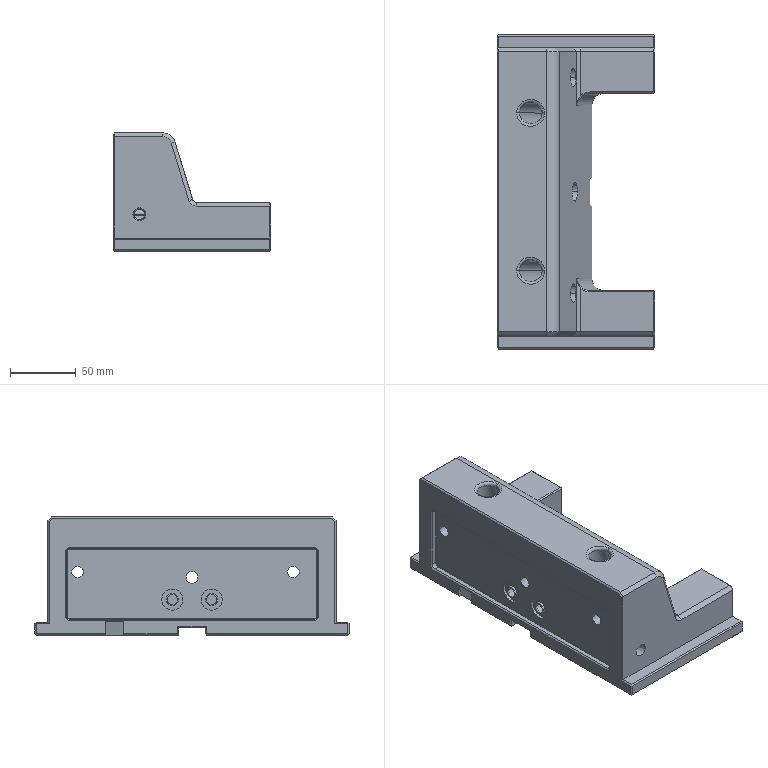Part | Creo | 1 solid | 249 faces | box 120 x 239 x 90 mm | volume 1168335 mm3 | plane 134 | cylinder 77 | cone 20 | spline 14 | torus 4 | commonest cylinder face diameters 8 x22 6 x10 14 x10 1.5 x8 9 x6 1 x4